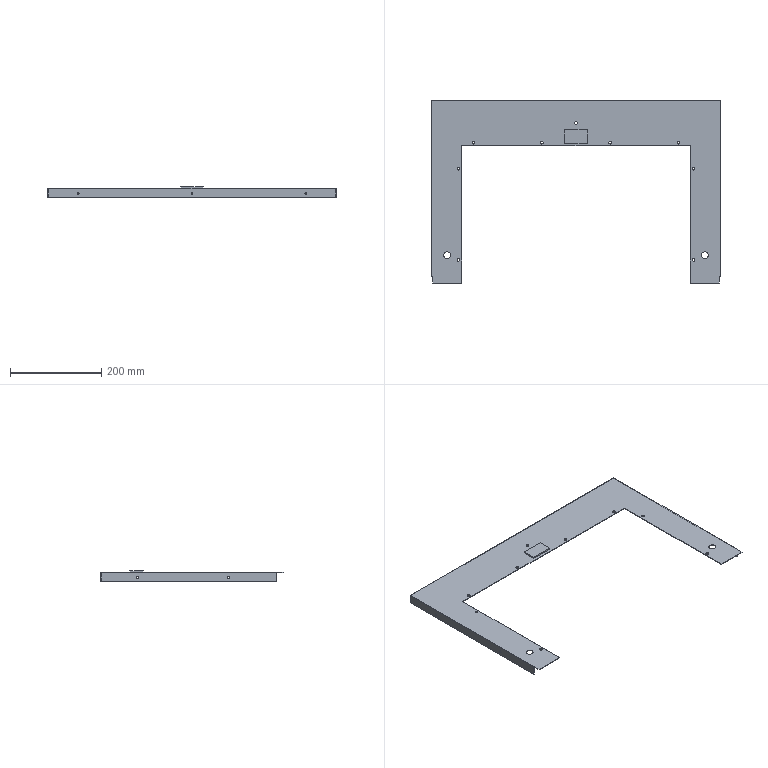Part | STEP file | 1 solid | 69 faces | box 632 x 399.5 x 23 mm | volume 156800 mm3 | cylinder 40 | plane 25 | cone 4 | commonest cylinder face diameters 6 x18 4.2 x14 3.3 x4 15 x4